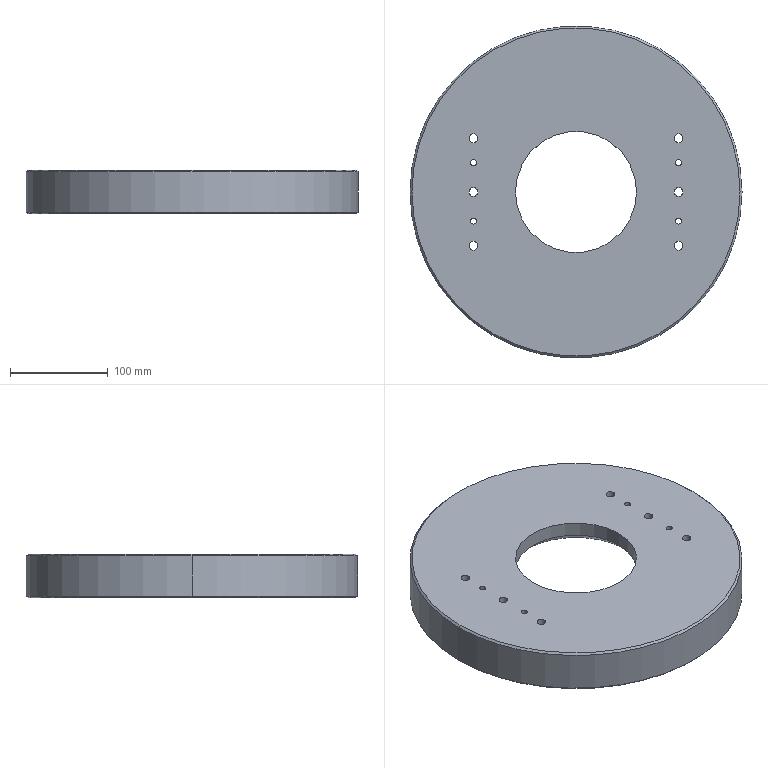Part | 1 solid | 64 faces | box 340 x 340 x 45 mm | volume 2483967 mm3 | cylinder 43 | cone 11 | plane 10 | commonest cylinder face diameters 9 x12 15 x12 6 x8 235 x5 124 x2 321 x2